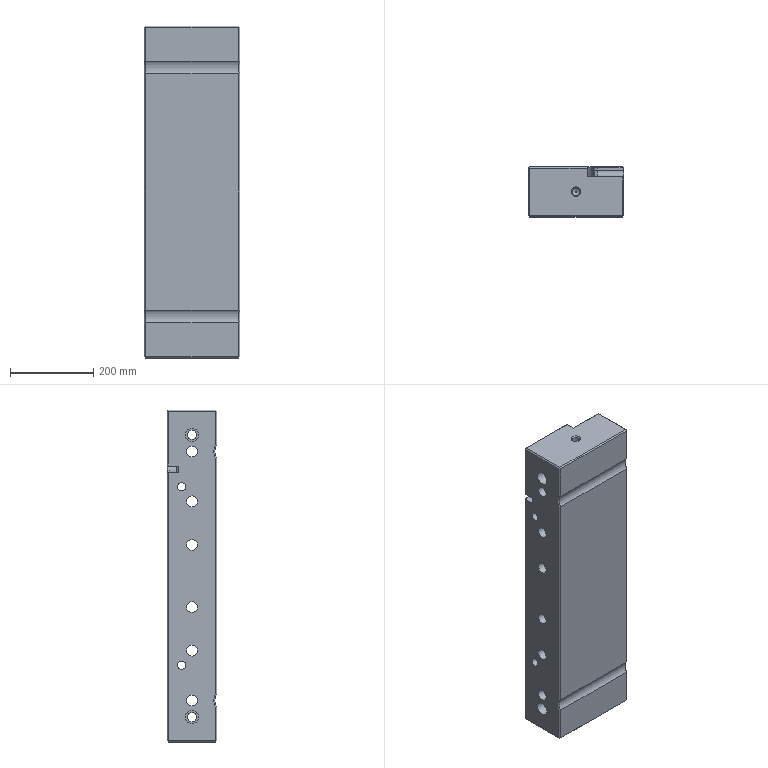Part | STEP file | solid 56 | 1 solid | 155 faces | box 230 x 120 x 800 mm | volume 20287508 mm3 | plane 92 | cylinder 38 | cone 24 | spline 1 | commonest cylinder face diameters 15 x8 26 x6 20 x5 4.2 x2 5 x2 10 x2